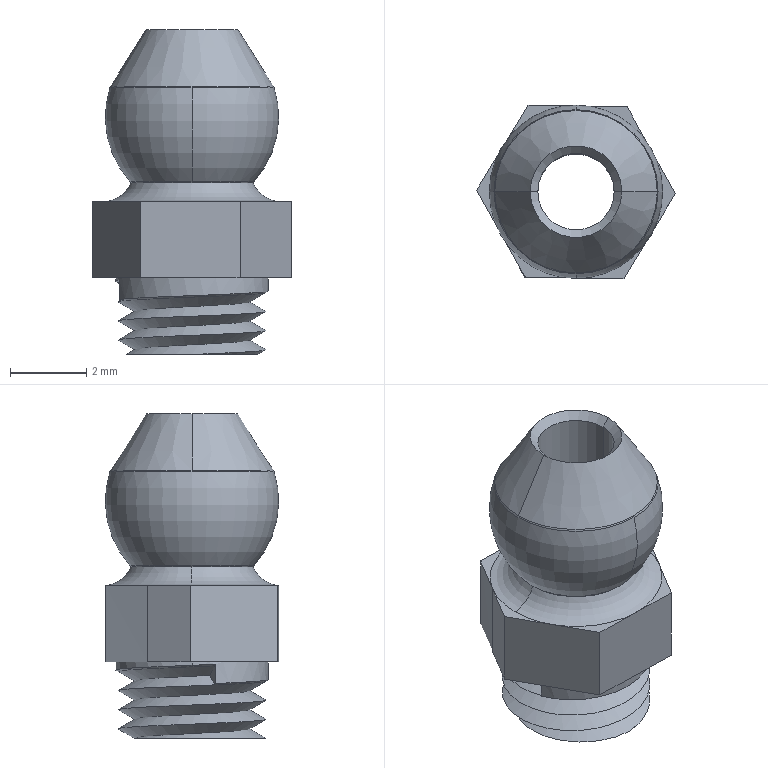Part | SolidWorks | features BaseBody 1 | 1 solid | 37 faces | box 5.195 x 4.548 x 8.5 mm | volume 81.788 mm3 | plane 16 | torus 8 | cylinder 5 | cone 4 | spline 4 | commonest cylinder face diameters 2 x2 4 x2 4.5 x1